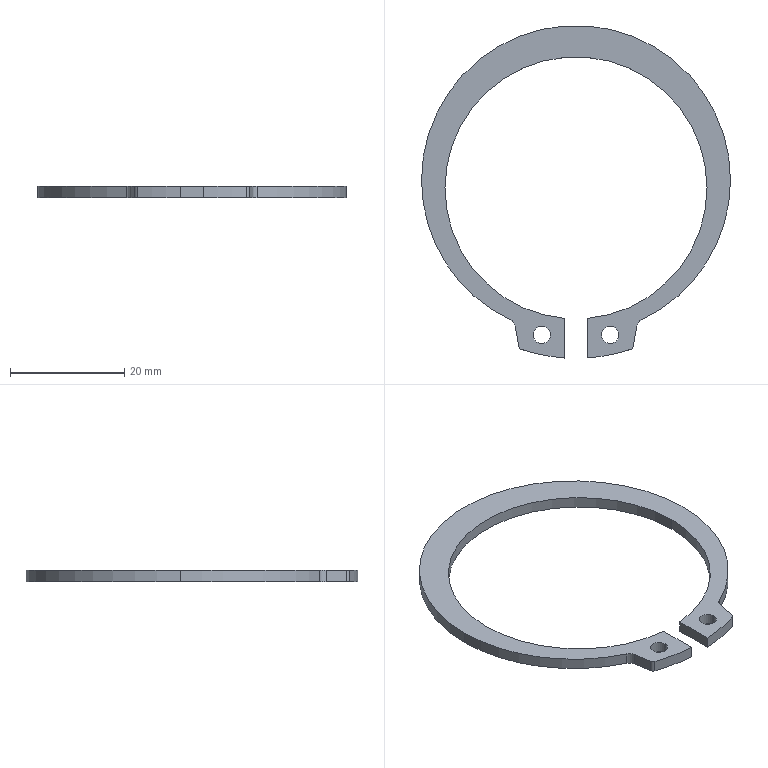Part | SolidWorks | features BaseBody 1 | 1 solid | 22 faces | box 54 x 58.103 x 2 mm | volume 1377 mm3 | cylinder 16 | plane 6 | commonest cylinder face diameters 3 x6 45.8 x3 54 x3 1.4 x2 59.6 x2
STEP:
#1=CARTESIAN_POINT('',(-27.,0.,1.));
#2=VERTEX_POINT('',#1);
#3=CARTESIAN_POINT('',(27.,0.,1.));
#4=VERTEX_POINT('',#3);
#5=CARTESIAN_POINT('',(0.,0.,1.));
#6=DIRECTION('',(0.,0.,-1.));
#7=DIRECTION('',(-1.,0.,0.));
#8=AXIS2_PLACEMENT_3D('',#5,#6,#7);
#9=CIRCLE('',#8,27.);
#10=EDGE_CURVE('',#2,#4,#9,.T.);
#11=ORIENTED_EDGE('',*,*,#10,.T.);
#12=CARTESIAN_POINT('',(27.,0.,-1.));
#13=VERTEX_POINT('',#12);
#14=CARTESIAN_POINT('',(27.,0.,1.));
#15=DIRECTION('',(0.,0.,-1.));
#16=VECTOR('',#15,1000.);
#17=LINE('',#14,#16);
#18=EDGE_CURVE('',#4,#13,#17,.T.);
#19=ORIENTED_EDGE('',*,*,#18,.T.);
#20=CARTESIAN_POINT('',(-27.,0.,-1.));
#21=VERTEX_POINT('',#20);
#22=CARTESIAN_POINT('',(0.,0.,-1.));
#23=DIRECTION('',(0.,0.,1.));
#24=DIRECTION('',(-1.,0.,0.));
#25=AXIS2_PLACEMENT_3D('',#22,#23,#24);
#26=CIRCLE('',#25,27.);
#27=EDGE_CURVE('',#13,#21,#26,.T.);
#28=ORIENTED_EDGE('',*,*,#27,.T.);
#29=CARTESIAN_POINT('',(-27.,0.,1.));
#30=DIRECTION('',(0.,0.,-1.));
#31=VECTOR('',#30,1000.);
#32=LINE('',#29,#31);
#33=EDGE_CURVE('',#2,#21,#32,.T.);
#34=ORIENTED_EDGE('',*,*,#33,.F.);
#35=EDGE_LOOP('',(#11,#19,#28,#34));
#36=FACE_OUTER_BOUND('',#35,.T.);
#37=CARTESIAN_POINT('',(0.,0.,1.));
#38=DIRECTION('',(0.,0.,-1.));
#39=DIRECTION('',(-1.,0.,0.));
#40=AXIS2_PLACEMENT_3D('',#37,#38,#39);
#41=CYLINDRICAL_SURFACE('',#40,27.);
#42=ADVANCED_FACE('',(#36),#41,.T.);
#43=CARTESIAN_POINT('',(-11.461,-24.447,1.));
#44=VERTEX_POINT('',#43);
#45=CARTESIAN_POINT('',(0.,0.,1.));
#46=DIRECTION('',(0.,0.,-1.));
#47=DIRECTION('',(-1.,0.,0.));
#48=AXIS2_PLACEMENT_3D('',#45,#46,#47);
#49=CIRCLE('',#48,27.);
#50=EDGE_CURVE('',#44,#2,#49,.T.);
#51=ORIENTED_EDGE('',*,*,#50,.T.);
#52=ORIENTED_EDGE('',*,*,#33,.T.);
#53=CARTESIAN_POINT('',(-11.461,-24.447,-1.));
#54=VERTEX_POINT('',#53);
#55=CARTESIAN_POINT('',(0.,0.,-1.));
#56=DIRECTION('',(0.,0.,1.));
#57=DIRECTION('',(-1.,0.,0.));
#58=AXIS2_PLACEMENT_3D('',#55,#56,#57);
#59=CIRCLE('',#58,27.);
#60=EDGE_CURVE('',#21,#54,#59,.T.);
#61=ORIENTED_EDGE('',*,*,#60,.T.);
#62=CARTESIAN_POINT('',(-11.461,-24.447,1.));
#63=DIRECTION('',(0.,0.,1.));
#64=VECTOR('',#63,1000.);
#65=LINE('',#62,#64);
#66=EDGE_CURVE('',#54,#44,#65,.T.);
#67=ORIENTED_EDGE('',*,*,#66,.T.);
#68=EDGE_LOOP('',(#51,#52,#61,#67));
#69=FACE_OUTER_BOUND('',#68,.T.);
#70=CARTESIAN_POINT('',(0.,0.,1.));
#71=DIRECTION('',(0.,0.,-1.));
#72=DIRECTION('',(-1.,0.,0.));
#73=AXIS2_PLACEMENT_3D('',#70,#71,#72);
#74=CYLINDRICAL_SURFACE('',#73,27.);
#75=ADVANCED_FACE('',(#69),#74,.T.);
#76=CARTESIAN_POINT('',(22.9,-1.37,1.));
#77=VERTEX_POINT('',#76);
#78=CARTESIAN_POINT('',(2.,-24.182,1.));
#79=VERTEX_POINT('',#78);
#80=CARTESIAN_POINT('',(0.,-1.37,1.));
#81=DIRECTION('',(0.,0.,-1.));
#82=DIRECTION('',(-1.,0.,0.));
#83=AXIS2_PLACEMENT_3D('',#80,#81,#82);
#84=CIRCLE('',#83,22.9);
#85=EDGE_CURVE('',#77,#79,#84,.T.);
#86=ORIENTED_EDGE('',*,*,#85,.F.);
#87=CARTESIAN_POINT('',(22.9,-1.37,-1.));
#88=VERTEX_POINT('',#87);
#89=CARTESIAN_POINT('',(22.9,-1.37,1.));
#90=DIRECTION('',(0.,0.,-1.));
#91=VECTOR('',#90,1000.);
#92=LINE('',#89,#91);
#93=EDGE_CURVE('',#77,#88,#92,.T.);
#94=ORIENTED_EDGE('',*,*,#93,.T.);
#95=CARTESIAN_POINT('',(2.,-24.182,-1.));
#96=VERTEX_POINT('',#95);
#97=CARTESIAN_POINT('',(0.,-1.37,-1.));
#98=DIRECTION('',(0.,0.,-1.));
#99=DIRECTION('',(-1.,0.,0.));
#100=AXIS2_PLACEMENT_3D('',#97,#98,#99);
#101=CIRCLE('',#100,22.9);
#102=EDGE_CURVE('',#88,#96,#101,.T.);
#103=ORIENTED_EDGE('',*,*,#102,.T.);
#104=CARTESIAN_POINT('',(2.,-24.182,1.));
#105=DIRECTION('',(0.,0.,1.));
#106=VECTOR('',#105,1000.);
#107=LINE('',#104,#106);
#108=EDGE_CURVE('',#96,#79,#107,.T.);
#109=ORIENTED_EDGE('',*,*,#108,.T.);
#110=EDGE_LOOP('',(#86,#94,#103,#109));
#111=FACE_OUTER_BOUND('',#110,.T.);
#112=CARTESIAN_POINT('',(0.,-1.37,1.));
#113=DIRECTION('',(0.,0.,-1.));
#114=DIRECTION('',(-1.,0.,0.));
#115=AXIS2_PLACEMENT_3D('',#112,#113,#114);
#116=CYLINDRICAL_SURFACE('',#115,22.9);
#117=ADVANCED_FACE('',(#111),#116,.F.);
#118=ORIENTED_EDGE('',*,*,#93,.F.);
#119=CARTESIAN_POINT('',(-22.9,-1.37,1.));
#120=VERTEX_POINT('',#119);
#121=CARTESIAN_POINT('',(0.,-1.37,1.));
#122=DIRECTION('',(0.,0.,-1.));
#123=DIRECTION('',(-1.,0.,0.));
#124=AXIS2_PLACEMENT_3D('',#121,#122,#123);
#125=CIRCLE('',#124,22.9);
#126=EDGE_CURVE('',#120,#77,#125,.T.);
#127=ORIENTED_EDGE('',*,*,#126,.F.);
#128=CARTESIAN_POINT('',(-22.9,-1.37,-1.));
#129=VERTEX_POINT('',#128);
#130=CARTESIAN_POINT('',(-22.9,-1.37,1.));
#131=DIRECTION('',(0.,0.,-1.));
#132=VECTOR('',#131,1000.);
#133=LINE('',#130,#132);
#134=EDGE_CURVE('',#120,#129,#133,.T.);
#135=ORIENTED_EDGE('',*,*,#134,.T.);
#136=CARTESIAN_POINT('',(0.,-1.37,-1.));
#137=DIRECTION('',(0.,0.,-1.));
#138=DIRECTION('',(-1.,0.,0.));
#139=AXIS2_PLACEMENT_3D('',#136,#137,#138);
#140=CIRCLE('',#139,22.9);
#141=EDGE_CURVE('',#129,#88,#140,.T.);
#142=ORIENTED_EDGE('',*,*,#141,.T.);
#143=EDGE_LOOP('',(#118,#127,#135,#142));
#144=FACE_OUTER_BOUND('',#143,.T.);
#145=CARTESIAN_POINT('',(0.,-1.37,1.));
#146=DIRECTION('',(0.,0.,-1.));
#147=DIRECTION('',(-1.,0.,0.));
#148=AXIS2_PLACEMENT_3D('',#145,#146,#147);
#149=CYLINDRICAL_SURFACE('',#148,22.9);
#150=ADVANCED_FACE('',(#144),#149,.F.);
#151=CARTESIAN_POINT('',(-4.5,-27.079,1.));
#152=VERTEX_POINT('',#151);
#153=CARTESIAN_POINT('',(-7.5,-27.079,1.));
#154=VERTEX_POINT('',#153);
#155=CARTESIAN_POINT('',(-6.,-27.079,1.));
#156=DIRECTION('',(0.,0.,-1.));
#157=DIRECTION('',(-1.,0.,0.));
#158=AXIS2_PLACEMENT_3D('',#155,#156,#157);
#159=CIRCLE('',#158,1.5);
#160=EDGE_CURVE('',#152,#154,#159,.T.);
#161=ORIENTED_EDGE('',*,*,#160,.F.);
#162=CARTESIAN_POINT('',(-4.5,-27.079,-1.));
#163=VERTEX_POINT('',#162);
#164=CARTESIAN_POINT('',(-4.5,-27.079,1.));
#165=DIRECTION('',(0.,0.,-1.));
#166=VECTOR('',#165,1000.);
#167=LINE('',#164,#166);
#168=EDGE_CURVE('',#152,#163,#167,.T.);
#169=ORIENTED_EDGE('',*,*,#168,.T.);
#170=CARTESIAN_POINT('',(-7.5,-27.079,-1.));
#171=VERTEX_POINT('',#170);
#172=CARTESIAN_POINT('',(-6.,-27.079,-1.));
#173=DIRECTION('',(0.,0.,-1.));
#174=DIRECTION('',(-1.,0.,0.));
#175=AXIS2_PLACEMENT_3D('',#172,#173,#174);
#176=CIRCLE('',#175,1.5);
#177=EDGE_CURVE('',#163,#171,#176,.T.);
#178=ORIENTED_EDGE('',*,*,#177,.T.);
#179=CARTESIAN_POINT('',(-7.5,-27.079,1.));
#180=DIRECTION('',(0.,0.,-1.));
#181=VECTOR('',#180,1000.);
#182=LINE('',#179,#181);
#183=EDGE_CURVE('',#154,#171,#182,.T.);
#184=ORIENTED_EDGE('',*,*,#183,.F.);
#185=EDGE_LOOP('',(#161,#169,#178,#184));
#186=FACE_OUTER_BOUND('',#185,.T.);
#187=CARTESIAN_POINT('',(-6.,-27.079,1.));
#188=DIRECTION('',(0.,0.,-1.));
#189=DIRECTION('',(-1.,0.,0.));
#190=AXIS2_PLACEMENT_3D('',#187,#188,#189);
#191=CYLINDRICAL_SURFACE('',#190,1.5);
#192=ADVANCED_FACE('',(#186),#191,.F.);
#193=CARTESIAN_POINT('',(7.5,-27.079,1.));
#194=VERTEX_POINT('',#193);
#195=CARTESIAN_POINT('',(4.5,-27.079,1.));
#196=VERTEX_POINT('',#195);
#197=CARTESIAN_POINT('',(6.,-27.079,1.));
#198=DIRECTION('',(0.,0.,-1.));
#199=DIRECTION('',(-1.,0.,0.));
#200=AXIS2_PLACEMENT_3D('',#197,#198,#199);
#201=CIRCLE('',#200,1.5);
#202=EDGE_CURVE('',#194,#196,#201,.T.);
#203=ORIENTED_EDGE('',*,*,#202,.F.);
#204=CARTESIAN_POINT('',(7.5,-27.079,-1.));
#205=VERTEX_POINT('',#204);
#206=CARTESIAN_POINT('',(7.5,-27.079,1.));
#207=DIRECTION('',(0.,0.,-1.));
#208=VECTOR('',#207,1000.);
#209=LINE('',#206,#208);
#210=EDGE_CURVE('',#194,#205,#209,.T.);
#211=ORIENTED_EDGE('',*,*,#210,.T.);
#212=CARTESIAN_POINT('',(4.5,-27.079,-1.));
#213=VERTEX_POINT('',#212);
#214=CARTESIAN_POINT('',(6.,-27.079,-1.));
#215=DIRECTION('',(0.,0.,-1.));
#216=DIRECTION('',(-1.,0.,0.));
#217=AXIS2_PLACEMENT_3D('',#214,#215,#216);
#218=CIRCLE('',#217,1.5);
#219=EDGE_CURVE('',#205,#213,#218,.T.);
#220=ORIENTED_EDGE('',*,*,#219,.T.);
#221=CARTESIAN_POINT('',(4.5,-27.079,1.));
#222=DIRECTION('',(0.,0.,-1.));
#223=VECTOR('',#222,1000.);
#224=LINE('',#221,#223);
#225=EDGE_CURVE('',#196,#213,#224,.T.);
#226=ORIENTED_EDGE('',*,*,#225,.F.);
#227=EDGE_LOOP('',(#203,#211,#220,#226));
#228=FACE_OUTER_BOUND('',#227,.T.);
#229=CARTESIAN_POINT('',(6.,-27.079,1.));
#230=DIRECTION('',(0.,0.,-1.));
#231=DIRECTION('',(-1.,0.,0.));
#232=AXIS2_PLACEMENT_3D('',#229,#230,#231);
#233=CYLINDRICAL_SURFACE('',#232,1.5);
#234=ADVANCED_FACE('',(#228),#233,.F.);
#235=CARTESIAN_POINT('',(-10.62,-25.545,-1.));
#236=VERTEX_POINT('',#235);
#237=CARTESIAN_POINT('',(-12.097,-25.805,-1.));
#238=DIRECTION('',(0.,0.,1.));
#239=DIRECTION('',(-1.,0.,0.));
#240=AXIS2_PLACEMENT_3D('',#237,#238,#239);
#241=CIRCLE('',#240,1.5);
#242=EDGE_CURVE('',#236,#54,#241,.T.);
#243=ORIENTED_EDGE('',*,*,#242,.T.);
#244=ORIENTED_EDGE('',*,*,#60,.F.);
#245=ORIENTED_EDGE('',*,*,#27,.F.);
#246=CARTESIAN_POINT('',(11.461,-24.447,-1.));
#247=VERTEX_POINT('',#246);
#248=CARTESIAN_POINT('',(0.,0.,-1.));
#249=DIRECTION('',(0.,0.,1.));
#250=DIRECTION('',(-1.,0.,0.));
#251=AXIS2_PLACEMENT_3D('',#248,#249,#250);
#252=CIRCLE('',#251,27.);
#253=EDGE_CURVE('',#247,#13,#252,.T.);
#254=ORIENTED_EDGE('',*,*,#253,.F.);
#255=CARTESIAN_POINT('',(10.62,-25.545,-1.));
#256=VERTEX_POINT('',#255);
#257=CARTESIAN_POINT('',(12.097,-25.805,-1.));
#258=DIRECTION('',(0.,0.,1.));
#259=DIRECTION('',(-1.,0.,0.));
#260=AXIS2_PLACEMENT_3D('',#257,#258,#259);
#261=CIRCLE('',#260,1.5);
#262=EDGE_CURVE('',#247,#256,#261,.T.);
#263=ORIENTED_EDGE('',*,*,#262,.T.);
#264=CARTESIAN_POINT('',(10.,-29.062,-1.));
#265=VERTEX_POINT('',#264);
#266=CARTESIAN_POINT('',(10.,-29.062,-1.));
#267=DIRECTION('',(0.1736,0.9848,0.));
#268=VECTOR('',#267,1000.);
#269=LINE('',#266,#268);
#270=EDGE_CURVE('',#265,#256,#269,.T.);
#271=ORIENTED_EDGE('',*,*,#270,.F.);
#272=CARTESIAN_POINT('',(9.535,-29.604,-1.));
#273=VERTEX_POINT('',#272);
#274=CARTESIAN_POINT('',(9.311,-28.94,-1.));
#275=DIRECTION('',(0.,0.,1.));
#276=DIRECTION('',(-1.,0.,0.));
#277=AXIS2_PLACEMENT_3D('',#274,#275,#276);
#278=CIRCLE('',#277,0.7);
#279=EDGE_CURVE('',#273,#265,#278,.T.);
#280=ORIENTED_EDGE('',*,*,#279,.F.);
#281=CARTESIAN_POINT('',(2.,-31.103,-1.));
#282=VERTEX_POINT('',#281);
#283=CARTESIAN_POINT('',(0.,-1.37,-1.));
#284=DIRECTION('',(0.,0.,1.));
#285=DIRECTION('',(-1.,0.,0.));
#286=AXIS2_PLACEMENT_3D('',#283,#284,#285);
#287=CIRCLE('',#286,29.8);
#288=EDGE_CURVE('',#282,#273,#287,.T.);
#289=ORIENTED_EDGE('',*,*,#288,.F.);
#290=CARTESIAN_POINT('',(2.,-25.805,-1.));
#291=DIRECTION('',(0.,-1.,0.));
#292=VECTOR('',#291,1000.);
#293=LINE('',#290,#292);
#294=EDGE_CURVE('',#96,#282,#293,.T.);
#295=ORIENTED_EDGE('',*,*,#294,.F.);
#296=ORIENTED_EDGE('',*,*,#102,.F.);
#297=ORIENTED_EDGE('',*,*,#141,.F.);
#298=CARTESIAN_POINT('',(-2.,-24.182,-1.));
#299=VERTEX_POINT('',#298);
#300=CARTESIAN_POINT('',(0.,-1.37,-1.));
#301=DIRECTION('',(0.,0.,-1.));
#302=DIRECTION('',(-1.,0.,0.));
#303=AXIS2_PLACEMENT_3D('',#300,#301,#302);
#304=CIRCLE('',#303,22.9);
#305=EDGE_CURVE('',#299,#129,#304,.T.);
#306=ORIENTED_EDGE('',*,*,#305,.F.);
#307=CARTESIAN_POINT('',(-2.,-31.103,-1.));
#308=VERTEX_POINT('',#307);
#309=CARTESIAN_POINT('',(-2.,-25.805,-1.));
#310=DIRECTION('',(0.,1.,0.));
#311=VECTOR('',#310,1000.);
#312=LINE('',#309,#311);
#313=EDGE_CURVE('',#308,#299,#312,.T.);
#314=ORIENTED_EDGE('',*,*,#313,.F.);
#315=CARTESIAN_POINT('',(-9.535,-29.604,-1.));
#316=VERTEX_POINT('',#315);
#317=CARTESIAN_POINT('',(0.,-1.37,-1.));
#318=DIRECTION('',(0.,0.,1.));
#319=DIRECTION('',(-1.,0.,0.));
#320=AXIS2_PLACEMENT_3D('',#317,#318,#319);
#321=CIRCLE('',#320,29.8);
#322=EDGE_CURVE('',#316,#308,#321,.T.);
#323=ORIENTED_EDGE('',*,*,#322,.F.);
#324=CARTESIAN_POINT('',(-10.,-29.062,-1.));
#325=VERTEX_POINT('',#324);
#326=CARTESIAN_POINT('',(-9.311,-28.94,-1.));
#327=DIRECTION('',(0.,0.,1.));
#328=DIRECTION('',(-1.,0.,0.));
#329=AXIS2_PLACEMENT_3D('',#326,#327,#328);
#330=CIRCLE('',#329,0.7);
#331=EDGE_CURVE('',#325,#316,#330,.T.);
#332=ORIENTED_EDGE('',*,*,#331,.F.);
#333=CARTESIAN_POINT('',(-10.62,-25.545,-1.));
#334=DIRECTION('',(0.1736,-0.9848,0.));
#335=VECTOR('',#334,1000.);
#336=LINE('',#333,#335);
#337=EDGE_CURVE('',#236,#325,#336,.T.);
#338=ORIENTED_EDGE('',*,*,#337,.F.);
#339=EDGE_LOOP('',(#243,#244,#245,#254,#263,#271,#280,#289,#295,#296,#297,#306,#314,#323,#332,#338));
#340=FACE_OUTER_BOUND('',#339,.T.);
#341=CARTESIAN_POINT('',(-6.,-27.079,-1.));
#342=DIRECTION('',(0.,0.,-1.));
#343=DIRECTION('',(-1.,0.,0.));
#344=AXIS2_PLACEMENT_3D('',#341,#342,#343);
#345=CIRCLE('',#344,1.5);
#346=EDGE_CURVE('',#171,#163,#345,.T.);
#347=ORIENTED_EDGE('',*,*,#346,.F.);
#348=ORIENTED_EDGE('',*,*,#177,.F.);
#349=EDGE_LOOP('',(#347,#348));
#350=FACE_BOUND('',#349,.T.);
#351=CARTESIAN_POINT('',(6.,-27.079,-1.));
#352=DIRECTION('',(0.,0.,-1.));
#353=DIRECTION('',(-1.,0.,0.));
#354=AXIS2_PLACEMENT_3D('',#351,#352,#353);
#355=CIRCLE('',#354,1.5);
#356=EDGE_CURVE('',#213,#205,#355,.T.);
#357=ORIENTED_EDGE('',*,*,#356,.F.);
#358=ORIENTED_EDGE('',*,*,#219,.F.);
#359=EDGE_LOOP('',(#357,#358));
#360=FACE_BOUND('',#359,.T.);
#361=CARTESIAN_POINT('',(-12.097,-25.805,-1.));
#362=DIRECTION('',(0.,0.,1.));
#363=DIRECTION('',(1.,0.,0.));
#364=AXIS2_PLACEMENT_3D('',#361,#362,#363);
#365=PLANE('',#364);
#366=ADVANCED_FACE('',(#340,#350,#360),#365,.F.);
#367=ORIENTED_EDGE('',*,*,#18,.F.);
#368=CARTESIAN_POINT('',(11.461,-24.447,1.));
#369=VERTEX_POINT('',#368);
#370=CARTESIAN_POINT('',(0.,0.,1.));
#371=DIRECTION('',(0.,0.,-1.));
#372=DIRECTION('',(-1.,0.,0.));
#373=AXIS2_PLACEMENT_3D('',#370,#371,#372);
#374=CIRCLE('',#373,27.);
#375=EDGE_CURVE('',#4,#369,#374,.T.);
#376=ORIENTED_EDGE('',*,*,#375,.T.);
#377=CARTESIAN_POINT('',(11.461,-24.447,1.));
#378=DIRECTION('',(0.,0.,-1.));
#379=VECTOR('',#378,1000.);
#380=LINE('',#377,#379);
#381=EDGE_CURVE('',#369,#247,#380,.T.);
#382=ORIENTED_EDGE('',*,*,#381,.T.);
#383=ORIENTED_EDGE('',*,*,#253,.T.);
#384=EDGE_LOOP('',(#367,#376,#382,#383));
#385=FACE_OUTER_BOUND('',#384,.T.);
#386=CARTESIAN_POINT('',(0.,0.,1.));
#387=DIRECTION('',(0.,0.,-1.));
#388=DIRECTION('',(-1.,0.,0.));
#389=AXIS2_PLACEMENT_3D('',#386,#387,#388);
#390=CYLINDRICAL_SURFACE('',#389,27.);
#391=ADVANCED_FACE('',(#385),#390,.T.);
#392=ORIENTED_EDGE('',*,*,#270,.T.);
#393=CARTESIAN_POINT('',(10.62,-25.545,1.));
#394=VERTEX_POINT('',#393);
#395=CARTESIAN_POINT('',(10.62,-25.545,1.));
#396=DIRECTION('',(0.,0.,-1.));
#397=VECTOR('',#396,1000.);
#398=LINE('',#395,#397);
#399=EDGE_CURVE('',#394,#256,#398,.T.);
#400=ORIENTED_EDGE('',*,*,#399,.F.);
#401=CARTESIAN_POINT('',(10.,-29.062,1.));
#402=VERTEX_POINT('',#401);
#403=CARTESIAN_POINT('',(10.62,-25.545,1.));
#404=DIRECTION('',(0.1736,0.9848,0.));
#405=VECTOR('',#404,1000.);
#406=LINE('',#403,#405);
#407=EDGE_CURVE('',#402,#394,#406,.T.);
#408=ORIENTED_EDGE('',*,*,#407,.F.);
#409=CARTESIAN_POINT('',(10.,-29.062,1.));
#410=DIRECTION('',(0.,0.,1.));
#411=VECTOR('',#410,1000.);
#412=LINE('',#409,#411);
#413=EDGE_CURVE('',#265,#402,#412,.T.);
#414=ORIENTED_EDGE('',*,*,#413,.F.);
#415=EDGE_LOOP('',(#392,#400,#408,#414));
#416=FACE_OUTER_BOUND('',#415,.T.);
#417=CARTESIAN_POINT('',(10.62,-25.545,1.));
#418=DIRECTION('',(-0.9848,0.1736,0.));
#419=DIRECTION('',(-0.1736,-0.9848,0.));
#420=AXIS2_PLACEMENT_3D('',#417,#418,#419);
#421=PLANE('',#420);
#422=ADVANCED_FACE('',(#416),#421,.F.);
#423=CARTESIAN_POINT('',(9.535,-29.604,1.));
#424=VERTEX_POINT('',#423);
#425=CARTESIAN_POINT('',(9.535,-29.604,1.));
#426=DIRECTION('',(0.,0.,1.));
#427=VECTOR('',#426,1000.);
#428=LINE('',#425,#427);
#429=EDGE_CURVE('',#273,#424,#428,.T.);
#430=ORIENTED_EDGE('',*,*,#429,.T.);
#431=CARTESIAN_POINT('',(2.,-31.103,1.));
#432=VERTEX_POINT('',#431);
#433=CARTESIAN_POINT('',(0.,-1.37,1.));
#434=DIRECTION('',(0.,0.,-1.));
#435=DIRECTION('',(-1.,0.,0.));
#436=AXIS2_PLACEMENT_3D('',#433,#434,#435);
#437=CIRCLE('',#436,29.8);
#438=EDGE_CURVE('',#424,#432,#437,.T.);
#439=ORIENTED_EDGE('',*,*,#438,.T.);
#440=CARTESIAN_POINT('',(2.,-31.103,1.));
#441=DIRECTION('',(0.,0.,-1.));
#442=VECTOR('',#441,1000.);
#443=LINE('',#440,#442);
#444=EDGE_CURVE('',#432,#282,#443,.T.);
#445=ORIENTED_EDGE('',*,*,#444,.T.);
#446=ORIENTED_EDGE('',*,*,#288,.T.);
#447=EDGE_LOOP('',(#430,#439,#445,#446));
#448=FACE_OUTER_BOUND('',#447,.T.);
#449=CARTESIAN_POINT('',(0.,-1.37,1.));
#450=DIRECTION('',(0.,0.,-1.));
#451=DIRECTION('',(-1.,0.,0.));
#452=AXIS2_PLACEMENT_3D('',#449,#450,#451);
#453=CYLINDRICAL_SURFACE('',#452,29.8);
#454=ADVANCED_FACE('',(#448),#453,.T.);
#455=ORIENTED_EDGE('',*,*,#294,.T.);
#456=ORIENTED_EDGE('',*,*,#444,.F.);
#457=CARTESIAN_POINT('',(2.,-24.182,1.));
#458=DIRECTION('',(0.,-1.,0.));
#459=VECTOR('',#458,1000.);
#460=LINE('',#457,#459);
#461=EDGE_CURVE('',#79,#432,#460,.T.);
#462=ORIENTED_EDGE('',*,*,#461,.F.);
#463=ORIENTED_EDGE('',*,*,#108,.F.);
#464=EDGE_LOOP('',(#455,#456,#462,#463));
#465=FACE_OUTER_BOUND('',#464,.T.);
#466=CARTESIAN_POINT('',(2.,-24.182,1.));
#467=DIRECTION('',(1.,0.,0.));
#468=DIRECTION('',(0.,1.,0.));
#469=AXIS2_PLACEMENT_3D('',#466,#467,#468);
#470=PLANE('',#469);
#471=ADVANCED_FACE('',(#465),#470,.F.);
#472=ORIENTED_EDGE('',*,*,#134,.F.);
#473=CARTESIAN_POINT('',(-2.,-24.182,1.));
#474=VERTEX_POINT('',#473);
#475=CARTESIAN_POINT('',(0.,-1.37,1.));
#476=DIRECTION('',(0.,0.,-1.));
#477=DIRECTION('',(-1.,0.,0.));
#478=AXIS2_PLACEMENT_3D('',#475,#476,#477);
#479=CIRCLE('',#478,22.9);
#480=EDGE_CURVE('',#474,#120,#479,.T.);
#481=ORIENTED_EDGE('',*,*,#480,.F.);
#482=CARTESIAN_POINT('',(-2.,-24.182,1.));
#483=DIRECTION('',(0.,0.,1.));
#484=VECTOR('',#483,1000.);
#485=LINE('',#482,#484);
#486=EDGE_CURVE('',#299,#474,#485,.T.);
#487=ORIENTED_EDGE('',*,*,#486,.F.);
#488=ORIENTED_EDGE('',*,*,#305,.T.);
#489=EDGE_LOOP('',(#472,#481,#487,#488));
#490=FACE_OUTER_BOUND('',#489,.T.);
#491=CARTESIAN_POINT('',(0.,-1.37,1.));
#492=DIRECTION('',(0.,0.,-1.));
#493=DIRECTION('',(-1.,0.,0.));
#494=AXIS2_PLACEMENT_3D('',#491,#492,#493);
#495=CYLINDRICAL_SURFACE('',#494,22.9);
#496=ADVANCED_FACE('',(#490),#495,.F.);
#497=ORIENTED_EDGE('',*,*,#313,.T.);
#498=ORIENTED_EDGE('',*,*,#486,.T.);
#499=CARTESIAN_POINT('',(-2.,-31.103,1.));
#500=VERTEX_POINT('',#499);
#501=CARTESIAN_POINT('',(-2.,-24.182,1.));
#502=DIRECTION('',(0.,1.,0.));
#503=VECTOR('',#502,1000.);
#504=LINE('',#501,#503);
#505=EDGE_CURVE('',#500,#474,#504,.T.);
#506=ORIENTED_EDGE('',*,*,#505,.F.);
#507=CARTESIAN_POINT('',(-2.,-31.103,1.));
#508=DIRECTION('',(0.,0.,1.));
#509=VECTOR('',#508,1000.);
#510=LINE('',#507,#509);
#511=EDGE_CURVE('',#308,#500,#510,.T.);
#512=ORIENTED_EDGE('',*,*,#511,.F.);
#513=EDGE_LOOP('',(#497,#498,#506,#512));
#514=FACE_OUTER_BOUND('',#513,.T.);
#515=CARTESIAN_POINT('',(-2.,-24.182,1.));
#516=DIRECTION('',(-1.,0.,0.));
#517=DIRECTION('',(0.,-1.,0.));
#518=AXIS2_PLACEMENT_3D('',#515,#516,#517);
#519=PLANE('',#518);
#520=ADVANCED_FACE('',(#514),#519,.F.);
#521=ORIENTED_EDGE('',*,*,#511,.T.);
#522=CARTESIAN_POINT('',(-9.535,-29.604,1.));
#523=VERTEX_POINT('',#522);
#524=CARTESIAN_POINT('',(0.,-1.37,1.));
#525=DIRECTION('',(0.,0.,-1.));
#526=DIRECTION('',(-1.,0.,0.));
#527=AXIS2_PLACEMENT_3D('',#524,#525,#526);
#528=CIRCLE('',#527,29.8);
#529=EDGE_CURVE('',#500,#523,#528,.T.);
#530=ORIENTED_EDGE('',*,*,#529,.T.);
#531=CARTESIAN_POINT('',(-9.535,-29.604,1.));
#532=DIRECTION('',(0.,0.,-1.));
#533=VECTOR('',#532,1000.);
#534=LINE('',#531,#533);
#535=EDGE_CURVE('',#523,#316,#534,.T.);
#536=ORIENTED_EDGE('',*,*,#535,.T.);
#537=ORIENTED_EDGE('',*,*,#322,.T.);
#538=EDGE_LOOP('',(#521,#530,#536,#537));
#539=FACE_OUTER_BOUND('',#538,.T.);
#540=CARTESIAN_POINT('',(0.,-1.37,1.));
#541=DIRECTION('',(0.,0.,-1.));
#542=DIRECTION('',(-1.,0.,0.));
#543=AXIS2_PLACEMENT_3D('',#540,#541,#542);
#544=CYLINDRICAL_SURFACE('',#543,29.8);
#545=ADVANCED_FACE('',(#539),#544,.T.);
#546=ORIENTED_EDGE('',*,*,#337,.T.);
#547=CARTESIAN_POINT('',(-10.,-29.062,1.));
#548=VERTEX_POINT('',#547);
#549=CARTESIAN_POINT('',(-10.,-29.062,1.));
#550=DIRECTION('',(0.,0.,-1.));
#551=VECTOR('',#550,1000.);
#552=LINE('',#549,#551);
#553=EDGE_CURVE('',#548,#325,#552,.T.);
#554=ORIENTED_EDGE('',*,*,#553,.F.);
#555=CARTESIAN_POINT('',(-10.62,-25.545,1.));
#556=VERTEX_POINT('',#555);
#557=CARTESIAN_POINT('',(-10.62,-25.545,1.));
#558=DIRECTION('',(0.1736,-0.9848,0.));
#559=VECTOR('',#558,1000.);
#560=LINE('',#557,#559);
#561=EDGE_CURVE('',#556,#548,#560,.T.);
#562=ORIENTED_EDGE('',*,*,#561,.F.);
#563=CARTESIAN_POINT('',(-10.62,-25.545,1.));
#564=DIRECTION('',(0.,0.,1.));
#565=VECTOR('',#564,1000.);
#566=LINE('',#563,#565);
#567=EDGE_CURVE('',#236,#556,#566,.T.);
#568=ORIENTED_EDGE('',*,*,#567,.F.);
#569=EDGE_LOOP('',(#546,#554,#562,#568));
#570=FACE_OUTER_BOUND('',#569,.T.);
#571=CARTESIAN_POINT('',(-10.62,-25.545,1.));
#572=DIRECTION('',(0.9848,0.1736,0.));
#573=DIRECTION('',(-0.1736,0.9848,0.));
#574=AXIS2_PLACEMENT_3D('',#571,#572,#573);
#575=PLANE('',#574);
#576=ADVANCED_FACE('',(#570),#575,.F.);
#577=ORIENTED_EDGE('',*,*,#168,.F.);
#578=CARTESIAN_POINT('',(-6.,-27.079,1.));
#579=DIRECTION('',(0.,0.,-1.));
#580=DIRECTION('',(-1.,0.,0.));
#581=AXIS2_PLACEMENT_3D('',#578,#579,#580);
#582=CIRCLE('',#581,1.5);
#583=EDGE_CURVE('',#154,#152,#582,.T.);
#584=ORIENTED_EDGE('',*,*,#583,.F.);
#585=ORIENTED_EDGE('',*,*,#183,.T.);
#586=ORIENTED_EDGE('',*,*,#346,.T.);
#587=EDGE_LOOP('',(#577,#584,#585,#586));
#588=FACE_OUTER_BOUND('',#587,.T.);
#589=CARTESIAN_POINT('',(-6.,-27.079,1.));
#590=DIRECTION('',(0.,0.,-1.));
#591=DIRECTION('',(-1.,0.,0.));
#592=AXIS2_PLACEMENT_3D('',#589,#590,#591);
#593=CYLINDRICAL_SURFACE('',#592,1.5);
#594=ADVANCED_FACE('',(#588),#593,.F.);
#595=ORIENTED_EDGE('',*,*,#210,.F.);
#596=CARTESIAN_POINT('',(6.,-27.079,1.));
#597=DIRECTION('',(0.,0.,-1.));
#598=DIRECTION('',(-1.,0.,0.));
#599=AXIS2_PLACEMENT_3D('',#596,#597,#598);
#600=CIRCLE('',#599,1.5);
#601=EDGE_CURVE('',#196,#194,#600,.T.);
#602=ORIENTED_EDGE('',*,*,#601,.F.);
#603=ORIENTED_EDGE('',*,*,#225,.T.);
#604=ORIENTED_EDGE('',*,*,#356,.T.);
#605=EDGE_LOOP('',(#595,#602,#603,#604));
#606=FACE_OUTER_BOUND('',#605,.T.);
#607=CARTESIAN_POINT('',(6.,-27.079,1.));
#608=DIRECTION('',(0.,0.,-1.));
#609=DIRECTION('',(-1.,0.,0.));
#610=AXIS2_PLACEMENT_3D('',#607,#608,#609);
#611=CYLINDRICAL_SURFACE('',#610,1.5);
#612=ADVANCED_FACE('',(#606),#611,.F.);
#613=ORIENTED_EDGE('',*,*,#242,.F.);
#614=ORIENTED_EDGE('',*,*,#567,.T.);
#615=CARTESIAN_POINT('',(-12.097,-25.805,1.));
#616=DIRECTION('',(0.,0.,-1.));
#617=DIRECTION('',(-1.,0.,0.));
#618=AXIS2_PLACEMENT_3D('',#615,#616,#617);
#619=CIRCLE('',#618,1.5);
#620=EDGE_CURVE('',#44,#556,#619,.T.);
#621=ORIENTED_EDGE('',*,*,#620,.F.);
#622=ORIENTED_EDGE('',*,*,#66,.F.);
#623=EDGE_LOOP('',(#613,#614,#621,#622));
#624=FACE_OUTER_BOUND('',#623,.T.);
#625=CARTESIAN_POINT('',(-12.097,-25.805,1.));
#626=DIRECTION('',(0.,0.,-1.));
#627=DIRECTION('',(-1.,0.,0.));
#628=AXIS2_PLACEMENT_3D('',#625,#626,#627);
#629=CYLINDRICAL_SURFACE('',#628,1.5);
#630=ADVANCED_FACE('',(#624),#629,.F.);
#631=ORIENTED_EDGE('',*,*,#601,.T.);
#632=ORIENTED_EDGE('',*,*,#202,.T.);
#633=EDGE_LOOP('',(#631,#632));
#634=FACE_BOUND('',#633,.T.);
#635=CARTESIAN_POINT('',(12.097,-25.805,1.));
#636=DIRECTION('',(0.,0.,-1.));
#637=DIRECTION('',(-1.,0.,0.));
#638=AXIS2_PLACEMENT_3D('',#635,#636,#637);
#639=CIRCLE('',#638,1.5);
#640=EDGE_CURVE('',#394,#369,#639,.T.);
#641=ORIENTED_EDGE('',*,*,#640,.T.);
#642=ORIENTED_EDGE('',*,*,#375,.F.);
#643=ORIENTED_EDGE('',*,*,#10,.F.);
#644=ORIENTED_EDGE('',*,*,#50,.F.);
#645=ORIENTED_EDGE('',*,*,#620,.T.);
#646=ORIENTED_EDGE('',*,*,#561,.T.);
#647=CARTESIAN_POINT('',(-9.311,-28.94,1.));
#648=DIRECTION('',(0.,0.,1.));
#649=DIRECTION('',(-1.,0.,0.));
#650=AXIS2_PLACEMENT_3D('',#647,#648,#649);
#651=CIRCLE('',#650,0.7);
#652=EDGE_CURVE('',#548,#523,#651,.T.);
#653=ORIENTED_EDGE('',*,*,#652,.T.);
#654=ORIENTED_EDGE('',*,*,#529,.F.);
#655=ORIENTED_EDGE('',*,*,#505,.T.);
#656=ORIENTED_EDGE('',*,*,#480,.T.);
#657=ORIENTED_EDGE('',*,*,#126,.T.);
#658=ORIENTED_EDGE('',*,*,#85,.T.);
#659=ORIENTED_EDGE('',*,*,#461,.T.);
#660=ORIENTED_EDGE('',*,*,#438,.F.);
#661=CARTESIAN_POINT('',(9.311,-28.94,1.));
#662=DIRECTION('',(0.,0.,1.));
#663=DIRECTION('',(-1.,0.,0.));
#664=AXIS2_PLACEMENT_3D('',#661,#662,#663);
#665=CIRCLE('',#664,0.7);
#666=EDGE_CURVE('',#424,#402,#665,.T.);
#667=ORIENTED_EDGE('',*,*,#666,.T.);
#668=ORIENTED_EDGE('',*,*,#407,.T.);
#669=EDGE_LOOP('',(#641,#642,#643,#644,#645,#646,#653,#654,#655,#656,#657,#658,#659,#660,#667,#668));
#670=FACE_OUTER_BOUND('',#669,.T.);
#671=ORIENTED_EDGE('',*,*,#583,.T.);
#672=ORIENTED_EDGE('',*,*,#160,.T.);
#673=EDGE_LOOP('',(#671,#672));
#674=FACE_BOUND('',#673,.T.);
#675=CARTESIAN_POINT('',(-12.097,-25.805,1.));
#676=DIRECTION('',(0.,0.,1.));
#677=DIRECTION('',(1.,0.,0.));
#678=AXIS2_PLACEMENT_3D('',#675,#676,#677);
#679=PLANE('',#678);
#680=ADVANCED_FACE('',(#634,#670,#674),#679,.T.);
#681=ORIENTED_EDGE('',*,*,#262,.F.);
#682=ORIENTED_EDGE('',*,*,#381,.F.);
#683=ORIENTED_EDGE('',*,*,#640,.F.);
#684=ORIENTED_EDGE('',*,*,#399,.T.);
#685=EDGE_LOOP('',(#681,#682,#683,#684));
#686=FACE_OUTER_BOUND('',#685,.T.);
#687=CARTESIAN_POINT('',(12.097,-25.805,1.));
#688=DIRECTION('',(0.,0.,-1.));
#689=DIRECTION('',(-1.,0.,0.));
#690=AXIS2_PLACEMENT_3D('',#687,#688,#689);
#691=CYLINDRICAL_SURFACE('',#690,1.5);
#692=ADVANCED_FACE('',(#686),#691,.F.);
#693=ORIENTED_EDGE('',*,*,#413,.T.);
#694=ORIENTED_EDGE('',*,*,#666,.F.);
#695=ORIENTED_EDGE('',*,*,#429,.F.);
#696=ORIENTED_EDGE('',*,*,#279,.T.);
#697=EDGE_LOOP('',(#693,#694,#695,#696));
#698=FACE_OUTER_BOUND('',#697,.T.);
#699=CARTESIAN_POINT('',(9.311,-28.94,1.));
#700=DIRECTION('',(0.,0.,-1.));
#701=DIRECTION('',(-1.,0.,0.));
#702=AXIS2_PLACEMENT_3D('',#699,#700,#701);
#703=CYLINDRICAL_SURFACE('',#702,0.7);
#704=ADVANCED_FACE('',(#698),#703,.T.);
#705=ORIENTED_EDGE('',*,*,#535,.F.);
#706=ORIENTED_EDGE('',*,*,#652,.F.);
#707=ORIENTED_EDGE('',*,*,#553,.T.);
#708=ORIENTED_EDGE('',*,*,#331,.T.);
#709=EDGE_LOOP('',(#705,#706,#707,#708));
#710=FACE_OUTER_BOUND('',#709,.T.);
#711=CARTESIAN_POINT('',(-9.311,-28.94,1.));
#712=DIRECTION('',(0.,0.,-1.));
#713=DIRECTION('',(-1.,0.,0.));
#714=AXIS2_PLACEMENT_3D('',#711,#712,#713);
#715=CYLINDRICAL_SURFACE('',#714,0.7);
#716=ADVANCED_FACE('',(#710),#715,.T.);
#717=CLOSED_SHELL('',(#42,#75,#117,#150,#192,#234,#366,#391,#422,#454,#471,#496,#520,#545,#576,#594,#612,#630,#680,#692,#704,#716));
#718=MANIFOLD_SOLID_BREP('',#717);
#719=CARTESIAN_POINT('',(0.,0.,0.));
#720=DIRECTION('',(0.,0.,1.));
#721=DIRECTION('',(1.,0.,0.));
#722=AXIS2_PLACEMENT_3D('',#719,#720,#721);
#723=(LENGTH_UNIT()NAMED_UNIT(*)SI_UNIT(.MILLI.,.METRE.));
#724=UNCERTAINTY_MEASURE_WITH_UNIT(LENGTH_MEASURE(0.00001),#723,'','');
#725=(NAMED_UNIT(*)PLANE_ANGLE_UNIT()SI_UNIT($,.RADIAN.));
#726=(NAMED_UNIT(*)SI_UNIT($,.STERADIAN.)SOLID_ANGLE_UNIT());
#727=(GEOMETRIC_REPRESENTATION_CONTEXT(3)GLOBAL_UNCERTAINTY_ASSIGNED_CONTEXT((#724))GLOBAL_UNIT_ASSIGNED_CONTEXT((#723,#725,#726))REPRESENTATION_CONTEXT('',''));
#728=ADVANCED_BREP_SHAPE_REPRESENTATION('',(#718,#722),#727);